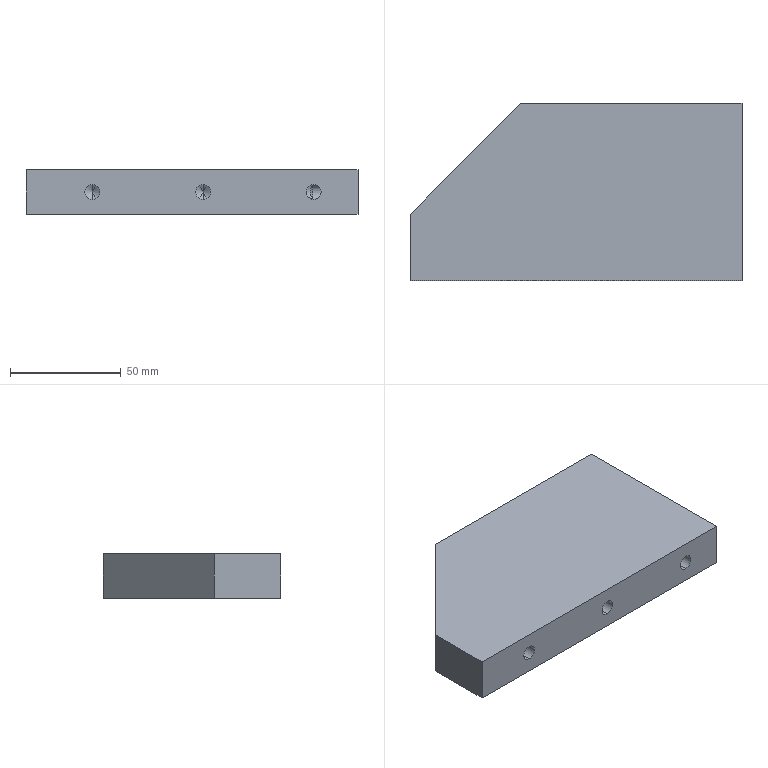Part | NX | features BREP 1 | 1 solid | 26 faces | box 150 x 80 x 20 mm | volume 211263 mm3 | cylinder 10 | cone 9 | plane 7 | commonest cylinder face diameters 6.8 x10
STEP:
#1=CARTESIAN_POINT('',(-45.,-19.5,13.4));
#2=VERTEX_POINT('',#1);
#3=CARTESIAN_POINT('',(-45.,-19.5,6.6));
#4=VERTEX_POINT('',#3);
#5=CARTESIAN_POINT('',(-45.,-19.5,10.));
#6=DIRECTION('',(0.,-1.,0.));
#7=DIRECTION('',(0.,0.,-1.));
#8=AXIS2_PLACEMENT_3D('',#5,#6,#7);
#9=CIRCLE('',#8,3.4);
#10=EDGE_CURVE('',#2,#4,#9,.T.);
#11=ORIENTED_EDGE('',*,*,#10,.F.);
#12=CARTESIAN_POINT('',(-45.,-40.,13.4));
#13=VERTEX_POINT('',#12);
#14=CARTESIAN_POINT('',(-45.,-40.,13.4));
#15=DIRECTION('',(0.,-1.,0.));
#16=VECTOR('',#15,1000.);
#17=LINE('',#14,#16);
#18=EDGE_CURVE('',#2,#13,#17,.T.);
#19=ORIENTED_EDGE('',*,*,#18,.T.);
#20=CARTESIAN_POINT('',(-45.,-40.,6.6));
#21=VERTEX_POINT('',#20);
#22=CARTESIAN_POINT('',(-45.,-40.,10.));
#23=DIRECTION('',(0.,-1.,0.));
#24=DIRECTION('',(0.,0.,-1.));
#25=AXIS2_PLACEMENT_3D('',#22,#23,#24);
#26=CIRCLE('',#25,3.4);
#27=EDGE_CURVE('',#13,#21,#26,.T.);
#28=ORIENTED_EDGE('',*,*,#27,.T.);
#29=CARTESIAN_POINT('',(-45.,-40.,6.6));
#30=DIRECTION('',(0.,-1.,0.));
#31=VECTOR('',#30,1000.);
#32=LINE('',#29,#31);
#33=EDGE_CURVE('',#4,#21,#32,.T.);
#34=ORIENTED_EDGE('',*,*,#33,.F.);
#35=EDGE_LOOP('',(#11,#19,#28,#34));
#36=FACE_BOUND('',#35,.T.);
#37=CARTESIAN_POINT('',(-45.,-40.,10.));
#38=DIRECTION('',(0.,-1.,0.));
#39=DIRECTION('',(0.,0.,-1.));
#40=AXIS2_PLACEMENT_3D('',#37,#38,#39);
#41=CYLINDRICAL_SURFACE('',#40,3.4);
#42=ADVANCED_FACE('',(#36),#41,.F.);
#43=CARTESIAN_POINT('',(-45.,-17.457,10.));
#44=VERTEX_POINT('',#43);
#45=CARTESIAN_POINT('',(-45.,-19.5,6.6));
#46=DIRECTION('',(0.,-0.515,-0.8572));
#47=VECTOR('',#46,1000.);
#48=LINE('',#45,#47);
#49=EDGE_CURVE('',#44,#4,#48,.T.);
#50=ORIENTED_EDGE('',*,*,#49,.F.);
#51=CARTESIAN_POINT('',(-45.,-19.5,13.4));
#52=DIRECTION('',(0.,-0.515,0.8572));
#53=VECTOR('',#52,1000.);
#54=LINE('',#51,#53);
#55=EDGE_CURVE('',#44,#2,#54,.T.);
#56=ORIENTED_EDGE('',*,*,#55,.T.);
#57=ORIENTED_EDGE('',*,*,#10,.T.);
#58=EDGE_LOOP('',(#50,#56,#57));
#59=FACE_BOUND('',#58,.T.);
#60=CARTESIAN_POINT('',(-45.,-19.5,10.));
#61=DIRECTION('',(0.,-1.,0.));
#62=DIRECTION('',(0.,0.,-1.));
#63=AXIS2_PLACEMENT_3D('',#60,#61,#62);
#64=CONICAL_SURFACE('',#63,3.4,1.03);
#65=ADVANCED_FACE('',(#59),#64,.F.);
#66=CARTESIAN_POINT('',(5.,-19.5,13.4));
#67=VERTEX_POINT('',#66);
#68=CARTESIAN_POINT('',(5.,-19.5,6.6));
#69=VERTEX_POINT('',#68);
#70=CARTESIAN_POINT('',(5.,-19.5,10.));
#71=DIRECTION('',(0.,-1.,0.));
#72=DIRECTION('',(0.,0.,-1.));
#73=AXIS2_PLACEMENT_3D('',#70,#71,#72);
#74=CIRCLE('',#73,3.4);
#75=EDGE_CURVE('',#67,#69,#74,.T.);
#76=ORIENTED_EDGE('',*,*,#75,.F.);
#77=CARTESIAN_POINT('',(5.,-40.,13.4));
#78=VERTEX_POINT('',#77);
#79=CARTESIAN_POINT('',(5.,-40.,13.4));
#80=DIRECTION('',(0.,-1.,0.));
#81=VECTOR('',#80,1000.);
#82=LINE('',#79,#81);
#83=EDGE_CURVE('',#67,#78,#82,.T.);
#84=ORIENTED_EDGE('',*,*,#83,.T.);
#85=CARTESIAN_POINT('',(5.,-40.,6.6));
#86=VERTEX_POINT('',#85);
#87=CARTESIAN_POINT('',(5.,-40.,10.));
#88=DIRECTION('',(0.,-1.,0.));
#89=DIRECTION('',(0.,0.,-1.));
#90=AXIS2_PLACEMENT_3D('',#87,#88,#89);
#91=CIRCLE('',#90,3.4);
#92=EDGE_CURVE('',#78,#86,#91,.T.);
#93=ORIENTED_EDGE('',*,*,#92,.T.);
#94=CARTESIAN_POINT('',(5.,-40.,6.6));
#95=DIRECTION('',(0.,-1.,0.));
#96=VECTOR('',#95,1000.);
#97=LINE('',#94,#96);
#98=EDGE_CURVE('',#69,#86,#97,.T.);
#99=ORIENTED_EDGE('',*,*,#98,.F.);
#100=EDGE_LOOP('',(#76,#84,#93,#99));
#101=FACE_BOUND('',#100,.T.);
#102=CARTESIAN_POINT('',(5.,-40.,10.));
#103=DIRECTION('',(0.,-1.,0.));
#104=DIRECTION('',(0.,0.,-1.));
#105=AXIS2_PLACEMENT_3D('',#102,#103,#104);
#106=CYLINDRICAL_SURFACE('',#105,3.4);
#107=ADVANCED_FACE('',(#101),#106,.F.);
#108=CARTESIAN_POINT('',(5.,-17.457,10.));
#109=VERTEX_POINT('',#108);
#110=CARTESIAN_POINT('',(5.,-19.5,6.6));
#111=DIRECTION('',(0.,-0.515,-0.8572));
#112=VECTOR('',#111,1000.);
#113=LINE('',#110,#112);
#114=EDGE_CURVE('',#109,#69,#113,.T.);
#115=ORIENTED_EDGE('',*,*,#114,.F.);
#116=CARTESIAN_POINT('',(5.,-19.5,13.4));
#117=DIRECTION('',(0.,-0.515,0.8572));
#118=VECTOR('',#117,1000.);
#119=LINE('',#116,#118);
#120=EDGE_CURVE('',#109,#67,#119,.T.);
#121=ORIENTED_EDGE('',*,*,#120,.T.);
#122=ORIENTED_EDGE('',*,*,#75,.T.);
#123=EDGE_LOOP('',(#115,#121,#122));
#124=FACE_BOUND('',#123,.T.);
#125=CARTESIAN_POINT('',(5.,-19.5,10.));
#126=DIRECTION('',(0.,-1.,0.));
#127=DIRECTION('',(0.,0.,-1.));
#128=AXIS2_PLACEMENT_3D('',#125,#126,#127);
#129=CONICAL_SURFACE('',#128,3.4,1.03);
#130=ADVANCED_FACE('',(#124),#129,.F.);
#131=CARTESIAN_POINT('',(55.,-19.5,13.4));
#132=VERTEX_POINT('',#131);
#133=CARTESIAN_POINT('',(54.429,-19.5,6.648));
#134=VERTEX_POINT('',#133);
#135=CARTESIAN_POINT('',(55.,-19.5,10.));
#136=DIRECTION('',(0.,-1.,0.));
#137=DIRECTION('',(0.,0.,-1.));
#138=AXIS2_PLACEMENT_3D('',#135,#136,#137);
#139=CIRCLE('',#138,3.4);
#140=EDGE_CURVE('',#132,#134,#139,.T.);
#141=ORIENTED_EDGE('',*,*,#140,.F.);
#142=CARTESIAN_POINT('',(55.,-40.,13.4));
#143=VERTEX_POINT('',#142);
#144=CARTESIAN_POINT('',(55.,-40.,13.4));
#145=DIRECTION('',(0.,-1.,0.));
#146=VECTOR('',#145,1000.);
#147=LINE('',#144,#146);
#148=EDGE_CURVE('',#132,#143,#147,.T.);
#149=ORIENTED_EDGE('',*,*,#148,.T.);
#150=CARTESIAN_POINT('',(55.,-40.,6.6));
#151=VERTEX_POINT('',#150);
#152=CARTESIAN_POINT('',(55.,-40.,10.));
#153=DIRECTION('',(0.,-1.,0.));
#154=DIRECTION('',(0.,0.,-1.));
#155=AXIS2_PLACEMENT_3D('',#152,#153,#154);
#156=CIRCLE('',#155,3.4);
#157=EDGE_CURVE('',#143,#151,#156,.T.);
#158=ORIENTED_EDGE('',*,*,#157,.T.);
#159=CARTESIAN_POINT('',(55.,-20.852,6.6));
#160=VERTEX_POINT('',#159);
#161=CARTESIAN_POINT('',(55.,-40.,6.6));
#162=DIRECTION('',(0.,-1.,0.));
#163=VECTOR('',#162,1000.);
#164=LINE('',#161,#163);
#165=EDGE_CURVE('',#160,#151,#164,.T.);
#166=ORIENTED_EDGE('',*,*,#165,.F.);
#167=CARTESIAN_POINT('',(54.5,-20.984,6.637));
#168=VERTEX_POINT('',#167);
#169=CARTESIAN_POINT('',(55.,-20.852,6.6));
#170=CARTESIAN_POINT('',(54.831,-20.852,6.6));
#171=CARTESIAN_POINT('',(54.67,-20.9,6.612));
#172=CARTESIAN_POINT('',(54.5,-20.984,6.637));
#173=B_SPLINE_CURVE_WITH_KNOTS('',3,(#169,#170,#171,#172),.UNSPECIFIED.,.F.,.F.,(4,4),(0.,1.),.UNSPECIFIED.);
#174=EDGE_CURVE('',#168,#160,#173,.F.);
#175=ORIENTED_EDGE('',*,*,#174,.F.);
#176=CARTESIAN_POINT('',(54.403,-20.,6.653));
#177=VERTEX_POINT('',#176);
#178=CARTESIAN_POINT('',(54.5,-20.984,6.637));
#179=CARTESIAN_POINT('',(54.435,-20.643,6.647));
#180=CARTESIAN_POINT('',(54.403,-20.315,6.653));
#181=CARTESIAN_POINT('',(54.403,-20.,6.653));
#182=B_SPLINE_CURVE_WITH_KNOTS('',3,(#178,#179,#180,#181),.UNSPECIFIED.,.F.,.F.,(4,4),(0.,1.),.UNSPECIFIED.);
#183=EDGE_CURVE('',#177,#168,#182,.F.);
#184=ORIENTED_EDGE('',*,*,#183,.F.);
#185=CARTESIAN_POINT('',(54.429,-19.5,6.648));
#186=CARTESIAN_POINT('',(54.412,-19.667,6.651));
#187=CARTESIAN_POINT('',(54.403,-19.833,6.653));
#188=CARTESIAN_POINT('',(54.403,-20.,6.653));
#189=B_SPLINE_CURVE_WITH_KNOTS('',3,(#185,#186,#187,#188),.UNSPECIFIED.,.F.,.F.,(4,4),(0.0003905,0.0008907),.UNSPECIFIED.);
#190=EDGE_CURVE('',#134,#177,#189,.T.);
#191=ORIENTED_EDGE('',*,*,#190,.F.);
#192=EDGE_LOOP('',(#141,#149,#158,#166,#175,#184,#191));
#193=FACE_BOUND('',#192,.T.);
#194=CARTESIAN_POINT('',(55.,-40.,10.));
#195=DIRECTION('',(0.,-1.,0.));
#196=DIRECTION('',(0.,0.,-1.));
#197=AXIS2_PLACEMENT_3D('',#194,#195,#196);
#198=CYLINDRICAL_SURFACE('',#197,3.4);
#199=ADVANCED_FACE('',(#193),#198,.F.);
#200=CARTESIAN_POINT('',(54.5,30.,13.292));
#201=VERTEX_POINT('',#200);
#202=CARTESIAN_POINT('',(54.5,30.,6.492));
#203=VERTEX_POINT('',#202);
#204=CARTESIAN_POINT('',(54.5,30.,9.892));
#205=DIRECTION('',(1.,0.,0.));
#206=DIRECTION('',(0.,0.,-1.));
#207=AXIS2_PLACEMENT_3D('',#204,#205,#206);
#208=CIRCLE('',#207,3.4);
#209=EDGE_CURVE('',#201,#203,#208,.T.);
#210=ORIENTED_EDGE('',*,*,#209,.F.);
#211=CARTESIAN_POINT('',(75.,30.,13.292));
#212=VERTEX_POINT('',#211);
#213=CARTESIAN_POINT('',(75.,30.,13.292));
#214=DIRECTION('',(1.,0.,0.));
#215=VECTOR('',#214,1000.);
#216=LINE('',#213,#215);
#217=EDGE_CURVE('',#201,#212,#216,.T.);
#218=ORIENTED_EDGE('',*,*,#217,.T.);
#219=CARTESIAN_POINT('',(75.,30.,6.492));
#220=VERTEX_POINT('',#219);
#221=CARTESIAN_POINT('',(75.,30.,9.892));
#222=DIRECTION('',(1.,0.,0.));
#223=DIRECTION('',(0.,0.,-1.));
#224=AXIS2_PLACEMENT_3D('',#221,#222,#223);
#225=CIRCLE('',#224,3.4);
#226=EDGE_CURVE('',#212,#220,#225,.T.);
#227=ORIENTED_EDGE('',*,*,#226,.T.);
#228=CARTESIAN_POINT('',(75.,30.,6.492));
#229=DIRECTION('',(1.,0.,0.));
#230=VECTOR('',#229,1000.);
#231=LINE('',#228,#230);
#232=EDGE_CURVE('',#203,#220,#231,.T.);
#233=ORIENTED_EDGE('',*,*,#232,.F.);
#234=EDGE_LOOP('',(#210,#218,#227,#233));
#235=FACE_BOUND('',#234,.T.);
#236=CARTESIAN_POINT('',(75.,30.,9.892));
#237=DIRECTION('',(1.,0.,0.));
#238=DIRECTION('',(0.,0.,-1.));
#239=AXIS2_PLACEMENT_3D('',#236,#237,#238);
#240=CYLINDRICAL_SURFACE('',#239,3.4);
#241=ADVANCED_FACE('',(#235),#240,.F.);
#242=CARTESIAN_POINT('',(52.457,30.,9.892));
#243=VERTEX_POINT('',#242);
#244=CARTESIAN_POINT('',(54.5,30.,6.492));
#245=DIRECTION('',(0.515,0.,-0.8572));
#246=VECTOR('',#245,1000.);
#247=LINE('',#244,#246);
#248=EDGE_CURVE('',#243,#203,#247,.T.);
#249=ORIENTED_EDGE('',*,*,#248,.F.);
#250=CARTESIAN_POINT('',(54.5,30.,13.292));
#251=DIRECTION('',(0.515,0.,0.8572));
#252=VECTOR('',#251,1000.);
#253=LINE('',#250,#252);
#254=EDGE_CURVE('',#243,#201,#253,.T.);
#255=ORIENTED_EDGE('',*,*,#254,.T.);
#256=ORIENTED_EDGE('',*,*,#209,.T.);
#257=EDGE_LOOP('',(#249,#255,#256));
#258=FACE_BOUND('',#257,.T.);
#259=CARTESIAN_POINT('',(54.5,30.,9.892));
#260=DIRECTION('',(1.,0.,0.));
#261=DIRECTION('',(0.,0.,-1.));
#262=AXIS2_PLACEMENT_3D('',#259,#260,#261);
#263=CONICAL_SURFACE('',#262,3.4,1.03);
#264=ADVANCED_FACE('',(#258),#263,.F.);
#265=ORIENTED_EDGE('',*,*,#174,.T.);
#266=CARTESIAN_POINT('',(55.852,-20.,13.292));
#267=VERTEX_POINT('',#266);
#268=CARTESIAN_POINT('',(55.,-20.852,6.6));
#269=CARTESIAN_POINT('',(55.236,-20.852,6.6));
#270=CARTESIAN_POINT('',(55.632,-21.038,6.65));
#271=CARTESIAN_POINT('',(55.962,-21.27,6.734));
#272=CARTESIAN_POINT('',(56.617,-21.781,6.965));
#273=CARTESIAN_POINT('',(57.125,-22.253,7.284));
#274=CARTESIAN_POINT('',(57.764,-22.838,7.983));
#275=CARTESIAN_POINT('',(58.075,-23.125,8.497));
#276=CARTESIAN_POINT('',(58.341,-23.364,9.228));
#277=CARTESIAN_POINT('',(58.422,-23.422,9.943));
#278=CARTESIAN_POINT('',(58.367,-23.345,10.652));
#279=CARTESIAN_POINT('',(58.121,-23.07,11.4));
#280=CARTESIAN_POINT('',(57.855,-22.784,11.882));
#281=CARTESIAN_POINT('',(57.46,-22.352,12.361));
#282=CARTESIAN_POINT('',(57.218,-22.087,12.582));
#283=CARTESIAN_POINT('',(56.879,-21.706,12.846));
#284=CARTESIAN_POINT('',(56.619,-21.409,13.));
#285=CARTESIAN_POINT('',(56.262,-20.955,13.16));
#286=CARTESIAN_POINT('',(56.041,-20.635,13.241));
#287=CARTESIAN_POINT('',(55.852,-20.233,13.292));
#288=CARTESIAN_POINT('',(55.852,-20.,13.292));
#289=B_SPLINE_CURVE_WITH_KNOTS('',3,(#268,#269,#270,#271,#272,#273,#274,#275,#276,#277,#278,#279,#280,#281,#282,#283,#284,#285,#286,#287,#288),.UNSPECIFIED.,.F.,.F.,(4,1,1,1,1,1,1,1,1,1,1,1,1,1,1,1,1,1,4),(0.,0.0625,0.09375,0.125,0.25,0.3125,0.375,0.4375,0.5,0.5625,0.625,0.6875,0.75,0.7812,0.8125,0.875,0.9062,0.9375,1.),.UNSPECIFIED.);
#290=EDGE_CURVE('',#160,#267,#289,.T.);
#291=ORIENTED_EDGE('',*,*,#290,.T.);
#292=CARTESIAN_POINT('',(75.,-20.,13.292));
#293=VERTEX_POINT('',#292);
#294=CARTESIAN_POINT('',(75.,-20.,13.292));
#295=DIRECTION('',(1.,0.,0.));
#296=VECTOR('',#295,1000.);
#297=LINE('',#294,#296);
#298=EDGE_CURVE('',#267,#293,#297,.T.);
#299=ORIENTED_EDGE('',*,*,#298,.T.);
#300=CARTESIAN_POINT('',(75.,-20.,6.492));
#301=VERTEX_POINT('',#300);
#302=CARTESIAN_POINT('',(75.,-20.,9.892));
#303=DIRECTION('',(1.,0.,0.));
#304=DIRECTION('',(0.,0.,-1.));
#305=AXIS2_PLACEMENT_3D('',#302,#303,#304);
#306=CIRCLE('',#305,3.4);
#307=EDGE_CURVE('',#293,#301,#306,.T.);
#308=ORIENTED_EDGE('',*,*,#307,.T.);
#309=CARTESIAN_POINT('',(54.5,-20.,6.492));
#310=VERTEX_POINT('',#309);
#311=CARTESIAN_POINT('',(75.,-20.,6.492));
#312=DIRECTION('',(1.,0.,0.));
#313=VECTOR('',#312,1000.);
#314=LINE('',#311,#313);
#315=EDGE_CURVE('',#310,#301,#314,.T.);
#316=ORIENTED_EDGE('',*,*,#315,.F.);
#317=CARTESIAN_POINT('',(54.5,-20.,9.892));
#318=DIRECTION('',(1.,0.,0.));
#319=DIRECTION('',(0.,0.,-1.));
#320=AXIS2_PLACEMENT_3D('',#317,#318,#319);
#321=CIRCLE('',#320,3.4);
#322=EDGE_CURVE('',#168,#310,#321,.T.);
#323=ORIENTED_EDGE('',*,*,#322,.F.);
#324=EDGE_LOOP('',(#265,#291,#299,#308,#316,#323));
#325=FACE_BOUND('',#324,.T.);
#326=CARTESIAN_POINT('',(75.,-20.,9.892));
#327=DIRECTION('',(1.,0.,0.));
#328=DIRECTION('',(0.,0.,-1.));
#329=AXIS2_PLACEMENT_3D('',#326,#327,#328);
#330=CYLINDRICAL_SURFACE('',#329,3.4);
#331=ADVANCED_FACE('',(#325),#330,.F.);
#332=ORIENTED_EDGE('',*,*,#190,.T.);
#333=CARTESIAN_POINT('',(54.5,-20.,6.492));
#334=DIRECTION('',(0.515,0.,-0.8572));
#335=VECTOR('',#334,1000.);
#336=LINE('',#333,#335);
#337=EDGE_CURVE('',#177,#310,#336,.T.);
#338=ORIENTED_EDGE('',*,*,#337,.T.);
#339=CARTESIAN_POINT('',(54.5,-19.429,13.243));
#340=VERTEX_POINT('',#339);
#341=CARTESIAN_POINT('',(54.5,-20.,9.892));
#342=DIRECTION('',(1.,0.,0.));
#343=DIRECTION('',(0.,0.,-1.));
#344=AXIS2_PLACEMENT_3D('',#341,#342,#343);
#345=CIRCLE('',#344,3.4);
#346=EDGE_CURVE('',#310,#340,#345,.T.);
#347=ORIENTED_EDGE('',*,*,#346,.T.);
#348=CARTESIAN_POINT('',(54.5,-19.429,13.243));
#349=CARTESIAN_POINT('',(54.348,-19.275,12.961));
#350=CARTESIAN_POINT('',(54.075,-18.993,12.409));
#351=CARTESIAN_POINT('',(53.791,-18.71,11.738));
#352=CARTESIAN_POINT('',(53.521,-18.435,10.859));
#353=CARTESIAN_POINT('',(53.327,-18.363,9.634));
#354=CARTESIAN_POINT('',(53.538,-18.625,8.609));
#355=CARTESIAN_POINT('',(53.862,-18.942,7.798));
#356=CARTESIAN_POINT('',(54.069,-19.145,7.337));
#357=CARTESIAN_POINT('',(54.276,-19.349,6.93));
#358=CARTESIAN_POINT('',(54.429,-19.5,6.648));
#359=B_SPLINE_CURVE_WITH_KNOTS('',3,(#348,#349,#350,#351,#352,#353,#354,#355,#356,#357,#358),.UNSPECIFIED.,.F.,.F.,(4,1,1,1,1,1,1,1,4),(0.,0.125,0.25,0.375,0.5,0.75,0.8125,0.875,1.),.UNSPECIFIED.);
#360=EDGE_CURVE('',#340,#134,#359,.T.);
#361=ORIENTED_EDGE('',*,*,#360,.T.);
#362=EDGE_LOOP('',(#332,#338,#347,#361));
#363=FACE_BOUND('',#362,.T.);
#364=CARTESIAN_POINT('',(54.5,-20.,9.892));
#365=DIRECTION('',(1.,0.,0.));
#366=DIRECTION('',(0.,0.,-1.));
#367=AXIS2_PLACEMENT_3D('',#364,#365,#366);
#368=CONICAL_SURFACE('',#367,3.4,1.03);
#369=ADVANCED_FACE('',(#363),#368,.F.);
#370=CARTESIAN_POINT('',(75.,-40.,0.));
#371=VERTEX_POINT('',#370);
#372=CARTESIAN_POINT('',(75.,40.,0.));
#373=VERTEX_POINT('',#372);
#374=CARTESIAN_POINT('',(75.,40.,0.));
#375=DIRECTION('',(0.,1.,0.));
#376=VECTOR('',#375,1000.);
#377=LINE('',#374,#376);
#378=EDGE_CURVE('',#371,#373,#377,.T.);
#379=ORIENTED_EDGE('',*,*,#378,.T.);
#380=CARTESIAN_POINT('',(75.,40.,20.));
#381=VERTEX_POINT('',#380);
#382=CARTESIAN_POINT('',(75.,40.,20.));
#383=DIRECTION('',(0.,0.,-1.));
#384=VECTOR('',#383,1000.);
#385=LINE('',#382,#384);
#386=EDGE_CURVE('',#381,#373,#385,.T.);
#387=ORIENTED_EDGE('',*,*,#386,.F.);
#388=CARTESIAN_POINT('',(75.,-40.,20.));
#389=VERTEX_POINT('',#388);
#390=CARTESIAN_POINT('',(75.,40.,20.));
#391=DIRECTION('',(0.,1.,0.));
#392=VECTOR('',#391,1000.);
#393=LINE('',#390,#392);
#394=EDGE_CURVE('',#389,#381,#393,.T.);
#395=ORIENTED_EDGE('',*,*,#394,.F.);
#396=CARTESIAN_POINT('',(75.,-40.,20.));
#397=DIRECTION('',(0.,0.,-1.));
#398=VECTOR('',#397,1000.);
#399=LINE('',#396,#398);
#400=EDGE_CURVE('',#389,#371,#399,.T.);
#401=ORIENTED_EDGE('',*,*,#400,.T.);
#402=EDGE_LOOP('',(#379,#387,#395,#401));
#403=FACE_BOUND('',#402,.T.);
#404=CARTESIAN_POINT('',(75.,30.,9.892));
#405=DIRECTION('',(1.,0.,0.));
#406=DIRECTION('',(0.,0.,-1.));
#407=AXIS2_PLACEMENT_3D('',#404,#405,#406);
#408=CIRCLE('',#407,3.4);
#409=EDGE_CURVE('',#220,#212,#408,.T.);
#410=ORIENTED_EDGE('',*,*,#409,.F.);
#411=ORIENTED_EDGE('',*,*,#226,.F.);
#412=EDGE_LOOP('',(#410,#411));
#413=FACE_BOUND('',#412,.T.);
#414=CARTESIAN_POINT('',(75.,-20.,9.892));
#415=DIRECTION('',(1.,0.,0.));
#416=DIRECTION('',(0.,0.,-1.));
#417=AXIS2_PLACEMENT_3D('',#414,#415,#416);
#418=CIRCLE('',#417,3.4);
#419=EDGE_CURVE('',#301,#293,#418,.T.);
#420=ORIENTED_EDGE('',*,*,#419,.F.);
#421=ORIENTED_EDGE('',*,*,#307,.F.);
#422=EDGE_LOOP('',(#420,#421));
#423=FACE_BOUND('',#422,.T.);
#424=CARTESIAN_POINT('',(75.,40.,20.));
#425=DIRECTION('',(-1.,0.,0.));
#426=DIRECTION('',(0.,0.,1.));
#427=AXIS2_PLACEMENT_3D('',#424,#425,#426);
#428=PLANE('',#427);
#429=ADVANCED_FACE('',(#403,#413,#423),#428,.F.);
#430=CARTESIAN_POINT('',(-25.,40.,0.));
#431=VERTEX_POINT('',#430);
#432=CARTESIAN_POINT('',(-75.,40.,0.));
#433=DIRECTION('',(-1.,0.,0.));
#434=VECTOR('',#433,1000.);
#435=LINE('',#432,#434);
#436=EDGE_CURVE('',#373,#431,#435,.T.);
#437=ORIENTED_EDGE('',*,*,#436,.T.);
#438=CARTESIAN_POINT('',(-25.,40.,20.));
#439=VERTEX_POINT('',#438);
#440=CARTESIAN_POINT('',(-25.,40.,20.));
#441=DIRECTION('',(0.,0.,1.));
#442=VECTOR('',#441,1000.);
#443=LINE('',#440,#442);
#444=EDGE_CURVE('',#431,#439,#443,.T.);
#445=ORIENTED_EDGE('',*,*,#444,.T.);
#446=CARTESIAN_POINT('',(-75.,40.,20.));
#447=DIRECTION('',(-1.,0.,0.));
#448=VECTOR('',#447,1000.);
#449=LINE('',#446,#448);
#450=EDGE_CURVE('',#381,#439,#449,.T.);
#451=ORIENTED_EDGE('',*,*,#450,.F.);
#452=ORIENTED_EDGE('',*,*,#386,.T.);
#453=EDGE_LOOP('',(#437,#445,#451,#452));
#454=FACE_BOUND('',#453,.T.);
#455=CARTESIAN_POINT('',(-75.,40.,20.));
#456=DIRECTION('',(0.,-1.,0.));
#457=DIRECTION('',(0.,0.,-1.));
#458=AXIS2_PLACEMENT_3D('',#455,#456,#457);
#459=PLANE('',#458);
#460=ADVANCED_FACE('',(#454),#459,.F.);
#461=CARTESIAN_POINT('',(-75.,-10.,20.));
#462=VERTEX_POINT('',#461);
#463=CARTESIAN_POINT('',(-75.,-40.,20.));
#464=VERTEX_POINT('',#463);
#465=CARTESIAN_POINT('',(-75.,40.,20.));
#466=DIRECTION('',(0.,-1.,0.));
#467=VECTOR('',#466,1000.);
#468=LINE('',#465,#467);
#469=EDGE_CURVE('',#462,#464,#468,.T.);
#470=ORIENTED_EDGE('',*,*,#469,.F.);
#471=CARTESIAN_POINT('',(-75.,-10.,0.));
#472=VERTEX_POINT('',#471);
#473=CARTESIAN_POINT('',(-75.,-10.,20.));
#474=DIRECTION('',(0.,0.,-1.));
#475=VECTOR('',#474,1000.);
#476=LINE('',#473,#475);
#477=EDGE_CURVE('',#462,#472,#476,.T.);
#478=ORIENTED_EDGE('',*,*,#477,.T.);
#479=CARTESIAN_POINT('',(-75.,-40.,0.));
#480=VERTEX_POINT('',#479);
#481=CARTESIAN_POINT('',(-75.,40.,0.));
#482=DIRECTION('',(0.,-1.,0.));
#483=VECTOR('',#482,1000.);
#484=LINE('',#481,#483);
#485=EDGE_CURVE('',#472,#480,#484,.T.);
#486=ORIENTED_EDGE('',*,*,#485,.T.);
#487=CARTESIAN_POINT('',(-75.,-40.,20.));
#488=DIRECTION('',(0.,0.,-1.));
#489=VECTOR('',#488,1000.);
#490=LINE('',#487,#489);
#491=EDGE_CURVE('',#464,#480,#490,.T.);
#492=ORIENTED_EDGE('',*,*,#491,.F.);
#493=EDGE_LOOP('',(#470,#478,#486,#492));
#494=FACE_BOUND('',#493,.T.);
#495=CARTESIAN_POINT('',(-75.,40.,20.));
#496=DIRECTION('',(1.,0.,0.));
#497=DIRECTION('',(0.,1.,0.));
#498=AXIS2_PLACEMENT_3D('',#495,#496,#497);
#499=PLANE('',#498);
#500=ADVANCED_FACE('',(#494),#499,.F.);
#501=CARTESIAN_POINT('',(-75.,-40.,0.));
#502=DIRECTION('',(1.,0.,0.));
#503=VECTOR('',#502,1000.);
#504=LINE('',#501,#503);
#505=EDGE_CURVE('',#480,#371,#504,.T.);
#506=ORIENTED_EDGE('',*,*,#505,.T.);
#507=ORIENTED_EDGE('',*,*,#400,.F.);
#508=CARTESIAN_POINT('',(-75.,-40.,20.));
#509=DIRECTION('',(1.,0.,0.));
#510=VECTOR('',#509,1000.);
#511=LINE('',#508,#510);
#512=EDGE_CURVE('',#464,#389,#511,.T.);
#513=ORIENTED_EDGE('',*,*,#512,.F.);
#514=ORIENTED_EDGE('',*,*,#491,.T.);
#515=EDGE_LOOP('',(#506,#507,#513,#514));
#516=FACE_BOUND('',#515,.T.);
#517=CARTESIAN_POINT('',(-45.,-40.,10.));
#518=DIRECTION('',(0.,-1.,0.));
#519=DIRECTION('',(0.,0.,-1.));
#520=AXIS2_PLACEMENT_3D('',#517,#518,#519);
#521=CIRCLE('',#520,3.4);
#522=EDGE_CURVE('',#21,#13,#521,.T.);
#523=ORIENTED_EDGE('',*,*,#522,.F.);
#524=ORIENTED_EDGE('',*,*,#27,.F.);
#525=EDGE_LOOP('',(#523,#524));
#526=FACE_BOUND('',#525,.T.);
#527=CARTESIAN_POINT('',(5.,-40.,10.));
#528=DIRECTION('',(0.,-1.,0.));
#529=DIRECTION('',(0.,0.,-1.));
#530=AXIS2_PLACEMENT_3D('',#527,#528,#529);
#531=CIRCLE('',#530,3.4);
#532=EDGE_CURVE('',#86,#78,#531,.T.);
#533=ORIENTED_EDGE('',*,*,#532,.F.);
#534=ORIENTED_EDGE('',*,*,#92,.F.);
#535=EDGE_LOOP('',(#533,#534));
#536=FACE_BOUND('',#535,.T.);
#537=CARTESIAN_POINT('',(55.,-40.,10.));
#538=DIRECTION('',(0.,-1.,0.));
#539=DIRECTION('',(0.,0.,-1.));
#540=AXIS2_PLACEMENT_3D('',#537,#538,#539);
#541=CIRCLE('',#540,3.4);
#542=EDGE_CURVE('',#151,#143,#541,.T.);
#543=ORIENTED_EDGE('',*,*,#542,.F.);
#544=ORIENTED_EDGE('',*,*,#157,.F.);
#545=EDGE_LOOP('',(#543,#544));
#546=FACE_BOUND('',#545,.T.);
#547=CARTESIAN_POINT('',(-75.,-40.,20.));
#548=DIRECTION('',(0.,1.,0.));
#549=DIRECTION('',(1.,0.,0.));
#550=AXIS2_PLACEMENT_3D('',#547,#548,#549);
#551=PLANE('',#550);
#552=ADVANCED_FACE('',(#516,#526,#536,#546),#551,.F.);
#553=ORIENTED_EDGE('',*,*,#450,.T.);
#554=CARTESIAN_POINT('',(-32.5,32.5,20.));
#555=DIRECTION('',(-0.7071,-0.7071,0.));
#556=VECTOR('',#555,1000.);
#557=LINE('',#554,#556);
#558=EDGE_CURVE('',#439,#462,#557,.T.);
#559=ORIENTED_EDGE('',*,*,#558,.T.);
#560=ORIENTED_EDGE('',*,*,#469,.T.);
#561=ORIENTED_EDGE('',*,*,#512,.T.);
#562=ORIENTED_EDGE('',*,*,#394,.T.);
#563=EDGE_LOOP('',(#553,#559,#560,#561,#562));
#564=FACE_BOUND('',#563,.T.);
#565=CARTESIAN_POINT('',(0.,0.,20.));
#566=DIRECTION('',(0.,0.,1.));
#567=DIRECTION('',(1.,0.,0.));
#568=AXIS2_PLACEMENT_3D('',#565,#566,#567);
#569=PLANE('',#568);
#570=ADVANCED_FACE('',(#564),#569,.T.);
#571=ORIENTED_EDGE('',*,*,#485,.F.);
#572=CARTESIAN_POINT('',(-75.,-10.,0.));
#573=DIRECTION('',(0.7071,0.7071,0.));
#574=VECTOR('',#573,1000.);
#575=LINE('',#572,#574);
#576=EDGE_CURVE('',#472,#431,#575,.T.);
#577=ORIENTED_EDGE('',*,*,#576,.T.);
#578=ORIENTED_EDGE('',*,*,#436,.F.);
#579=ORIENTED_EDGE('',*,*,#378,.F.);
#580=ORIENTED_EDGE('',*,*,#505,.F.);
#581=EDGE_LOOP('',(#571,#577,#578,#579,#580));
#582=FACE_BOUND('',#581,.T.);
#583=CARTESIAN_POINT('',(0.,0.,0.));
#584=DIRECTION('',(0.,0.,1.));
#585=DIRECTION('',(1.,0.,0.));
#586=AXIS2_PLACEMENT_3D('',#583,#584,#585);
#587=PLANE('',#586);
#588=ADVANCED_FACE('',(#582),#587,.F.);
#589=ORIENTED_EDGE('',*,*,#337,.F.);
#590=ORIENTED_EDGE('',*,*,#183,.T.);
#591=ORIENTED_EDGE('',*,*,#322,.T.);
#592=EDGE_LOOP('',(#589,#590,#591));
#593=FACE_BOUND('',#592,.T.);
#594=CARTESIAN_POINT('',(54.5,-20.,9.892));
#595=DIRECTION('',(1.,0.,0.));
#596=DIRECTION('',(0.,0.,-1.));
#597=AXIS2_PLACEMENT_3D('',#594,#595,#596);
#598=CONICAL_SURFACE('',#597,3.4,1.03);
#599=ADVANCED_FACE('',(#593),#598,.F.);
#600=ORIENTED_EDGE('',*,*,#298,.F.);
#601=CARTESIAN_POINT('',(55.984,-19.5,13.255));
#602=VERTEX_POINT('',#601);
#603=CARTESIAN_POINT('',(55.852,-20.,13.292));
#604=CARTESIAN_POINT('',(55.852,-19.832,13.292));
#605=CARTESIAN_POINT('',(55.9,-19.67,13.28));
#606=CARTESIAN_POINT('',(55.984,-19.5,13.255));
#607=B_SPLINE_CURVE_WITH_KNOTS('',3,(#603,#604,#605,#606),.UNSPECIFIED.,.F.,.F.,(4,4),(0.,1.),.UNSPECIFIED.);
#608=EDGE_CURVE('',#267,#602,#607,.T.);
#609=ORIENTED_EDGE('',*,*,#608,.T.);
#610=CARTESIAN_POINT('',(55.984,-19.5,13.255));
#611=CARTESIAN_POINT('',(55.476,-19.404,13.24));
#612=CARTESIAN_POINT('',(55.003,-19.378,13.234));
#613=CARTESIAN_POINT('',(54.5,-19.429,13.243));
#614=B_SPLINE_CURVE_WITH_KNOTS('',3,(#610,#611,#612,#613),.UNSPECIFIED.,.F.,.F.,(4,4),(0.,1.),.UNSPECIFIED.);
#615=EDGE_CURVE('',#602,#340,#614,.T.);
#616=ORIENTED_EDGE('',*,*,#615,.T.);
#617=ORIENTED_EDGE('',*,*,#346,.F.);
#618=ORIENTED_EDGE('',*,*,#315,.T.);
#619=ORIENTED_EDGE('',*,*,#419,.T.);
#620=EDGE_LOOP('',(#600,#609,#616,#617,#618,#619));
#621=FACE_BOUND('',#620,.T.);
#622=CARTESIAN_POINT('',(75.,-20.,9.892));
#623=DIRECTION('',(1.,0.,0.));
#624=DIRECTION('',(0.,0.,-1.));
#625=AXIS2_PLACEMENT_3D('',#622,#623,#624);
#626=CYLINDRICAL_SURFACE('',#625,3.4);
#627=ADVANCED_FACE('',(#621),#626,.F.);
#628=ORIENTED_EDGE('',*,*,#254,.F.);
#629=ORIENTED_EDGE('',*,*,#248,.T.);
#630=CARTESIAN_POINT('',(54.5,30.,9.892));
#631=DIRECTION('',(1.,0.,0.));
#632=DIRECTION('',(0.,0.,-1.));
#633=AXIS2_PLACEMENT_3D('',#630,#631,#632);
#634=CIRCLE('',#633,3.4);
#635=EDGE_CURVE('',#203,#201,#634,.T.);
#636=ORIENTED_EDGE('',*,*,#635,.T.);
#637=EDGE_LOOP('',(#628,#629,#636));
#638=FACE_BOUND('',#637,.T.);
#639=CARTESIAN_POINT('',(54.5,30.,9.892));
#640=DIRECTION('',(1.,0.,0.));
#641=DIRECTION('',(0.,0.,-1.));
#642=AXIS2_PLACEMENT_3D('',#639,#640,#641);
#643=CONICAL_SURFACE('',#642,3.4,1.03);
#644=ADVANCED_FACE('',(#638),#643,.F.);
#645=ORIENTED_EDGE('',*,*,#217,.F.);
#646=ORIENTED_EDGE('',*,*,#635,.F.);
#647=ORIENTED_EDGE('',*,*,#232,.T.);
#648=ORIENTED_EDGE('',*,*,#409,.T.);
#649=EDGE_LOOP('',(#645,#646,#647,#648));
#650=FACE_BOUND('',#649,.T.);
#651=CARTESIAN_POINT('',(75.,30.,9.892));
#652=DIRECTION('',(1.,0.,0.));
#653=DIRECTION('',(0.,0.,-1.));
#654=AXIS2_PLACEMENT_3D('',#651,#652,#653);
#655=CYLINDRICAL_SURFACE('',#654,3.4);
#656=ADVANCED_FACE('',(#650),#655,.F.);
#657=ORIENTED_EDGE('',*,*,#148,.F.);
#658=CARTESIAN_POINT('',(55.,-19.5,10.));
#659=DIRECTION('',(0.,-1.,0.));
#660=DIRECTION('',(0.,0.,-1.));
#661=AXIS2_PLACEMENT_3D('',#658,#659,#660);
#662=CIRCLE('',#661,3.4);
#663=EDGE_CURVE('',#602,#132,#662,.T.);
#664=ORIENTED_EDGE('',*,*,#663,.F.);
#665=ORIENTED_EDGE('',*,*,#608,.F.);
#666=ORIENTED_EDGE('',*,*,#290,.F.);
#667=ORIENTED_EDGE('',*,*,#165,.T.);
#668=ORIENTED_EDGE('',*,*,#542,.T.);
#669=EDGE_LOOP('',(#657,#664,#665,#666,#667,#668));
#670=FACE_BOUND('',#669,.T.);
#671=CARTESIAN_POINT('',(55.,-40.,10.));
#672=DIRECTION('',(0.,-1.,0.));
#673=DIRECTION('',(0.,0.,-1.));
#674=AXIS2_PLACEMENT_3D('',#671,#672,#673);
#675=CYLINDRICAL_SURFACE('',#674,3.4);
#676=ADVANCED_FACE('',(#670),#675,.F.);
#677=ORIENTED_EDGE('',*,*,#615,.F.);
#678=ORIENTED_EDGE('',*,*,#663,.T.);
#679=ORIENTED_EDGE('',*,*,#140,.T.);
#680=ORIENTED_EDGE('',*,*,#360,.F.);
#681=EDGE_LOOP('',(#677,#678,#679,#680));
#682=FACE_BOUND('',#681,.T.);
#683=CARTESIAN_POINT('',(55.,-19.5,10.));
#684=DIRECTION('',(0.,-1.,0.));
#685=DIRECTION('',(0.,0.,-1.));
#686=AXIS2_PLACEMENT_3D('',#683,#684,#685);
#687=CONICAL_SURFACE('',#686,3.4,1.03);
#688=ADVANCED_FACE('',(#682),#687,.F.);
#689=ORIENTED_EDGE('',*,*,#120,.F.);
#690=ORIENTED_EDGE('',*,*,#114,.T.);
#691=CARTESIAN_POINT('',(5.,-19.5,10.));
#692=DIRECTION('',(0.,-1.,0.));
#693=DIRECTION('',(0.,0.,-1.));
#694=AXIS2_PLACEMENT_3D('',#691,#692,#693);
#695=CIRCLE('',#694,3.4);
#696=EDGE_CURVE('',#69,#67,#695,.T.);
#697=ORIENTED_EDGE('',*,*,#696,.T.);
#698=EDGE_LOOP('',(#689,#690,#697));
#699=FACE_BOUND('',#698,.T.);
#700=CARTESIAN_POINT('',(5.,-19.5,10.));
#701=DIRECTION('',(0.,-1.,0.));
#702=DIRECTION('',(0.,0.,-1.));
#703=AXIS2_PLACEMENT_3D('',#700,#701,#702);
#704=CONICAL_SURFACE('',#703,3.4,1.03);
#705=ADVANCED_FACE('',(#699),#704,.F.);
#706=ORIENTED_EDGE('',*,*,#83,.F.);
#707=ORIENTED_EDGE('',*,*,#696,.F.);
#708=ORIENTED_EDGE('',*,*,#98,.T.);
#709=ORIENTED_EDGE('',*,*,#532,.T.);
#710=EDGE_LOOP('',(#706,#707,#708,#709));
#711=FACE_BOUND('',#710,.T.);
#712=CARTESIAN_POINT('',(5.,-40.,10.));
#713=DIRECTION('',(0.,-1.,0.));
#714=DIRECTION('',(0.,0.,-1.));
#715=AXIS2_PLACEMENT_3D('',#712,#713,#714);
#716=CYLINDRICAL_SURFACE('',#715,3.4);
#717=ADVANCED_FACE('',(#711),#716,.F.);
#718=ORIENTED_EDGE('',*,*,#55,.F.);
#719=ORIENTED_EDGE('',*,*,#49,.T.);
#720=CARTESIAN_POINT('',(-45.,-19.5,10.));
#721=DIRECTION('',(0.,-1.,0.));
#722=DIRECTION('',(0.,0.,-1.));
#723=AXIS2_PLACEMENT_3D('',#720,#721,#722);
#724=CIRCLE('',#723,3.4);
#725=EDGE_CURVE('',#4,#2,#724,.T.);
#726=ORIENTED_EDGE('',*,*,#725,.T.);
#727=EDGE_LOOP('',(#718,#719,#726));
#728=FACE_BOUND('',#727,.T.);
#729=CARTESIAN_POINT('',(-45.,-19.5,10.));
#730=DIRECTION('',(0.,-1.,0.));
#731=DIRECTION('',(0.,0.,-1.));
#732=AXIS2_PLACEMENT_3D('',#729,#730,#731);
#733=CONICAL_SURFACE('',#732,3.4,1.03);
#734=ADVANCED_FACE('',(#728),#733,.F.);
#735=ORIENTED_EDGE('',*,*,#18,.F.);
#736=ORIENTED_EDGE('',*,*,#725,.F.);
#737=ORIENTED_EDGE('',*,*,#33,.T.);
#738=ORIENTED_EDGE('',*,*,#522,.T.);
#739=EDGE_LOOP('',(#735,#736,#737,#738));
#740=FACE_BOUND('',#739,.T.);
#741=CARTESIAN_POINT('',(-45.,-40.,10.));
#742=DIRECTION('',(0.,-1.,0.));
#743=DIRECTION('',(0.,0.,-1.));
#744=AXIS2_PLACEMENT_3D('',#741,#742,#743);
#745=CYLINDRICAL_SURFACE('',#744,3.4);
#746=ADVANCED_FACE('',(#740),#745,.F.);
#747=ORIENTED_EDGE('',*,*,#558,.F.);
#748=ORIENTED_EDGE('',*,*,#444,.F.);
#749=ORIENTED_EDGE('',*,*,#576,.F.);
#750=ORIENTED_EDGE('',*,*,#477,.F.);
#751=EDGE_LOOP('',(#747,#748,#749,#750));
#752=FACE_BOUND('',#751,.T.);
#753=CARTESIAN_POINT('',(-75.,-10.,20.));
#754=DIRECTION('',(0.7071,-0.7071,0.));
#755=DIRECTION('',(0.,0.,-1.));
#756=AXIS2_PLACEMENT_3D('',#753,#754,#755);
#757=PLANE('',#756);
#758=ADVANCED_FACE('',(#752),#757,.F.);
#759=CLOSED_SHELL('',(#42,#65,#107,#130,#199,#241,#264,#331,#369,#429,#460,#500,#552,#570,#588,#599,#627,#644,#656,#676,#688,#705,#717,#734,#746,#758));
#760=MANIFOLD_SOLID_BREP('',#759);
#761=(LENGTH_UNIT()NAMED_UNIT(*)SI_UNIT(.MILLI.,.METRE.));
#762=UNCERTAINTY_MEASURE_WITH_UNIT(LENGTH_MEASURE(0.0508),#761,'','');
#763=(NAMED_UNIT(*)PLANE_ANGLE_UNIT()SI_UNIT($,.RADIAN.));
#764=(NAMED_UNIT(*)SI_UNIT($,.STERADIAN.)SOLID_ANGLE_UNIT());
#765=(GEOMETRIC_REPRESENTATION_CONTEXT(3)GLOBAL_UNCERTAINTY_ASSIGNED_CONTEXT((#762))GLOBAL_UNIT_ASSIGNED_CONTEXT((#761,#763,#764))REPRESENTATION_CONTEXT('',''));
#766=ADVANCED_BREP_SHAPE_REPRESENTATION('',(#760),#765);